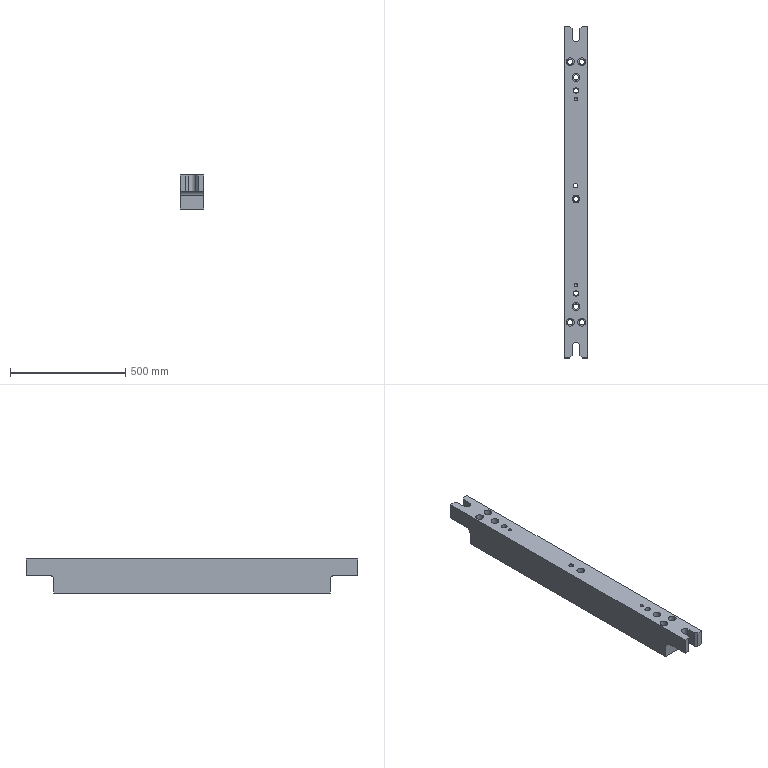Part | STEP file | lll_id2298_x_t | 1 solid | 56 faces | box 100 x 1440 x 147.5 mm | volume 18136196 mm3 | plane 29 | cylinder 25 | cone 2 | commonest cylinder face diameters 23.009 x7 34.008 x7 20 x3 14.506 x2 24 x2 34 x2
STEP:
#1=CARTESIAN_POINT('',(1317.435,-600.,222.5));
#2=VERTEX_POINT('',#1);
#3=CARTESIAN_POINT('',(1317.435,600.,222.5));
#4=VERTEX_POINT('',#3);
#5=CARTESIAN_POINT('',(1317.435,-1.,222.5));
#6=DIRECTION('',(0.,1.,0.));
#7=VECTOR('',#6,1.);
#8=LINE('',#5,#7);
#9=EDGE_CURVE('',#2,#4,#8,.T.);
#10=ORIENTED_EDGE('',*,*,#9,.T.);
#11=CARTESIAN_POINT('',(1417.435,600.,222.5));
#12=VERTEX_POINT('',#11);
#13=CARTESIAN_POINT('',(-848.88,600.,222.5));
#14=DIRECTION('',(1.,0.,0.));
#15=VECTOR('',#14,1.);
#16=LINE('',#13,#15);
#17=EDGE_CURVE('',#4,#12,#16,.T.);
#18=ORIENTED_EDGE('',*,*,#17,.T.);
#19=CARTESIAN_POINT('',(1417.435,-600.,222.5));
#20=VERTEX_POINT('',#19);
#21=CARTESIAN_POINT('',(1417.435,-1.,222.5));
#22=DIRECTION('',(0.,1.,0.));
#23=VECTOR('',#22,1.);
#24=LINE('',#21,#23);
#25=EDGE_CURVE('',#20,#12,#24,.T.);
#26=ORIENTED_EDGE('',*,*,#25,.F.);
#27=CARTESIAN_POINT('',(-848.88,-600.,222.5));
#28=DIRECTION('',(-1.,0.,0.));
#29=VECTOR('',#28,1.);
#30=LINE('',#27,#29);
#31=EDGE_CURVE('',#20,#2,#30,.T.);
#32=ORIENTED_EDGE('',*,*,#31,.T.);
#33=EDGE_LOOP('',(#10,#18,#26,#32));
#34=FACE_BOUND('',#33,.T.);
#35=CARTESIAN_POINT('',(1377.435,-440.,222.5));
#36=VERTEX_POINT('',#35);
#37=CARTESIAN_POINT('',(1367.435,-440.,222.5));
#38=DIRECTION('',(0.,0.,-1.));
#39=DIRECTION('',(1.,0.,0.));
#40=AXIS2_PLACEMENT_3D('',#37,#38,#39);
#41=CIRCLE('',#40,10.);
#42=EDGE_CURVE('',#36,#36,#41,.T.);
#43=ORIENTED_EDGE('',*,*,#42,.F.);
#44=EDGE_LOOP('',(#43));
#45=FACE_BOUND('',#44,.T.);
#46=CARTESIAN_POINT('',(1403.94,-565.,222.5));
#47=VERTEX_POINT('',#46);
#48=CARTESIAN_POINT('',(1392.435,-565.,222.5));
#49=DIRECTION('',(0.,0.,-1.));
#50=DIRECTION('',(1.,0.,0.));
#51=AXIS2_PLACEMENT_3D('',#48,#49,#50);
#52=CIRCLE('',#51,11.505);
#53=EDGE_CURVE('',#47,#47,#52,.T.);
#54=ORIENTED_EDGE('',*,*,#53,.F.);
#55=EDGE_LOOP('',(#54));
#56=FACE_BOUND('',#55,.T.);
#57=CARTESIAN_POINT('',(1353.94,-565.,222.5));
#58=VERTEX_POINT('',#57);
#59=CARTESIAN_POINT('',(1342.435,-565.,222.5));
#60=DIRECTION('',(0.,0.,-1.));
#61=DIRECTION('',(1.,0.,0.));
#62=AXIS2_PLACEMENT_3D('',#59,#60,#61);
#63=CIRCLE('',#62,11.505);
#64=EDGE_CURVE('',#58,#58,#63,.T.);
#65=ORIENTED_EDGE('',*,*,#64,.F.);
#66=EDGE_LOOP('',(#65));
#67=FACE_BOUND('',#66,.T.);
#68=CARTESIAN_POINT('',(1378.94,-497.,222.5));
#69=VERTEX_POINT('',#68);
#70=CARTESIAN_POINT('',(1367.435,-497.,222.5));
#71=DIRECTION('',(0.,0.,-1.));
#72=DIRECTION('',(1.,0.,0.));
#73=AXIS2_PLACEMENT_3D('',#70,#71,#72);
#74=CIRCLE('',#73,11.505);
#75=EDGE_CURVE('',#69,#69,#74,.T.);
#76=ORIENTED_EDGE('',*,*,#75,.F.);
#77=EDGE_LOOP('',(#76));
#78=FACE_BOUND('',#77,.T.);
#79=CARTESIAN_POINT('',(1378.94,-30.,222.5));
#80=VERTEX_POINT('',#79);
#81=CARTESIAN_POINT('',(1367.435,-30.,222.5));
#82=DIRECTION('',(0.,0.,-1.));
#83=DIRECTION('',(1.,0.,0.));
#84=AXIS2_PLACEMENT_3D('',#81,#82,#83);
#85=CIRCLE('',#84,11.505);
#86=EDGE_CURVE('',#80,#80,#85,.T.);
#87=ORIENTED_EDGE('',*,*,#86,.F.);
#88=EDGE_LOOP('',(#87));
#89=FACE_BOUND('',#88,.T.);
#90=CARTESIAN_POINT('',(1380.931,565.,222.5));
#91=VERTEX_POINT('',#90);
#92=CARTESIAN_POINT('',(1392.435,565.,222.5));
#93=DIRECTION('',(0.,0.,-1.));
#94=DIRECTION('',(-1.,0.,0.));
#95=AXIS2_PLACEMENT_3D('',#92,#93,#94);
#96=CIRCLE('',#95,11.505);
#97=EDGE_CURVE('',#91,#91,#96,.T.);
#98=ORIENTED_EDGE('',*,*,#97,.F.);
#99=EDGE_LOOP('',(#98));
#100=FACE_BOUND('',#99,.T.);
#101=CARTESIAN_POINT('',(1355.931,497.,222.5));
#102=VERTEX_POINT('',#101);
#103=CARTESIAN_POINT('',(1367.435,497.,222.5));
#104=DIRECTION('',(0.,0.,-1.));
#105=DIRECTION('',(-1.,0.,0.));
#106=AXIS2_PLACEMENT_3D('',#103,#104,#105);
#107=CIRCLE('',#106,11.505);
#108=EDGE_CURVE('',#102,#102,#107,.T.);
#109=ORIENTED_EDGE('',*,*,#108,.F.);
#110=EDGE_LOOP('',(#109));
#111=FACE_BOUND('',#110,.T.);
#112=CARTESIAN_POINT('',(1357.435,440.,222.5));
#113=VERTEX_POINT('',#112);
#114=CARTESIAN_POINT('',(1367.435,440.,222.5));
#115=DIRECTION('',(0.,0.,-1.));
#116=DIRECTION('',(-1.,0.,0.));
#117=AXIS2_PLACEMENT_3D('',#114,#115,#116);
#118=CIRCLE('',#117,10.);
#119=EDGE_CURVE('',#113,#113,#118,.T.);
#120=ORIENTED_EDGE('',*,*,#119,.F.);
#121=EDGE_LOOP('',(#120));
#122=FACE_BOUND('',#121,.T.);
#123=CARTESIAN_POINT('',(1330.931,565.,222.5));
#124=VERTEX_POINT('',#123);
#125=CARTESIAN_POINT('',(1342.435,565.,222.5));
#126=DIRECTION('',(0.,0.,-1.));
#127=DIRECTION('',(-1.,0.,0.));
#128=AXIS2_PLACEMENT_3D('',#125,#126,#127);
#129=CIRCLE('',#128,11.505);
#130=EDGE_CURVE('',#124,#124,#129,.T.);
#131=ORIENTED_EDGE('',*,*,#130,.F.);
#132=EDGE_LOOP('',(#131));
#133=FACE_BOUND('',#132,.T.);
#134=CARTESIAN_POINT('',(1376.,27.75,222.5));
#135=VERTEX_POINT('',#134);
#136=CARTESIAN_POINT('',(1366.,27.75,222.5));
#137=DIRECTION('',(0.,0.,1.));
#138=DIRECTION('',(1.,0.,0.));
#139=AXIS2_PLACEMENT_3D('',#136,#137,#138);
#140=CIRCLE('',#139,10.);
#141=EDGE_CURVE('',#135,#135,#140,.T.);
#142=ORIENTED_EDGE('',*,*,#141,.T.);
#143=EDGE_LOOP('',(#142));
#144=FACE_BOUND('',#143,.T.);
#145=CARTESIAN_POINT('',(-848.88,-1.,222.5));
#146=DIRECTION('',(0.,0.,-1.));
#147=DIRECTION('',(1.,0.,0.));
#148=AXIS2_PLACEMENT_3D('',#145,#146,#147);
#149=PLANE('',#148);
#150=ADVANCED_FACE('',(#34,#45,#56,#67,#78,#89,#100,#111,#122,#133,#144),#149,.T.);
#151=CARTESIAN_POINT('',(1356.,27.75,370.));
#152=VERTEX_POINT('',#151);
#153=CARTESIAN_POINT('',(1366.,27.75,370.));
#154=DIRECTION('',(0.,0.,-1.));
#155=DIRECTION('',(-1.,0.,0.));
#156=AXIS2_PLACEMENT_3D('',#153,#154,#155);
#157=CIRCLE('',#156,10.);
#158=EDGE_CURVE('',#152,#152,#157,.T.);
#159=ORIENTED_EDGE('',*,*,#158,.T.);
#160=EDGE_LOOP('',(#159));
#161=FACE_BOUND('',#160,.T.);
#162=CARTESIAN_POINT('',(1325.431,565.,370.));
#163=VERTEX_POINT('',#162);
#164=CARTESIAN_POINT('',(1342.435,565.,370.));
#165=DIRECTION('',(0.,0.,-1.));
#166=DIRECTION('',(-1.,0.,0.));
#167=AXIS2_PLACEMENT_3D('',#164,#165,#166);
#168=CIRCLE('',#167,17.004);
#169=EDGE_CURVE('',#163,#163,#168,.T.);
#170=ORIENTED_EDGE('',*,*,#169,.T.);
#171=EDGE_LOOP('',(#170));
#172=FACE_BOUND('',#171,.T.);
#173=CARTESIAN_POINT('',(1355.435,440.,370.));
#174=VERTEX_POINT('',#173);
#175=CARTESIAN_POINT('',(1367.435,440.,370.));
#176=DIRECTION('',(0.,0.,-1.));
#177=DIRECTION('',(-1.,0.,0.));
#178=AXIS2_PLACEMENT_3D('',#175,#176,#177);
#179=CIRCLE('',#178,12.);
#180=EDGE_CURVE('',#174,#174,#179,.T.);
#181=ORIENTED_EDGE('',*,*,#180,.T.);
#182=EDGE_LOOP('',(#181));
#183=FACE_BOUND('',#182,.T.);
#184=CARTESIAN_POINT('',(1350.431,497.,370.));
#185=VERTEX_POINT('',#184);
#186=CARTESIAN_POINT('',(1367.435,497.,370.));
#187=DIRECTION('',(0.,0.,-1.));
#188=DIRECTION('',(-1.,0.,0.));
#189=AXIS2_PLACEMENT_3D('',#186,#187,#188);
#190=CIRCLE('',#189,17.004);
#191=EDGE_CURVE('',#185,#185,#190,.T.);
#192=ORIENTED_EDGE('',*,*,#191,.T.);
#193=EDGE_LOOP('',(#192));
#194=FACE_BOUND('',#193,.T.);
#195=CARTESIAN_POINT('',(1375.431,565.,370.));
#196=VERTEX_POINT('',#195);
#197=CARTESIAN_POINT('',(1392.435,565.,370.));
#198=DIRECTION('',(0.,0.,-1.));
#199=DIRECTION('',(-1.,0.,0.));
#200=AXIS2_PLACEMENT_3D('',#197,#198,#199);
#201=CIRCLE('',#200,17.004);
#202=EDGE_CURVE('',#196,#196,#201,.T.);
#203=ORIENTED_EDGE('',*,*,#202,.T.);
#204=EDGE_LOOP('',(#203));
#205=FACE_BOUND('',#204,.T.);
#206=CARTESIAN_POINT('',(1384.439,-30.,370.));
#207=VERTEX_POINT('',#206);
#208=CARTESIAN_POINT('',(1367.435,-30.,370.));
#209=DIRECTION('',(0.,0.,-1.));
#210=DIRECTION('',(1.,0.,0.));
#211=AXIS2_PLACEMENT_3D('',#208,#209,#210);
#212=CIRCLE('',#211,17.004);
#213=EDGE_CURVE('',#207,#207,#212,.T.);
#214=ORIENTED_EDGE('',*,*,#213,.T.);
#215=EDGE_LOOP('',(#214));
#216=FACE_BOUND('',#215,.T.);
#217=CARTESIAN_POINT('',(1384.439,-497.,370.));
#218=VERTEX_POINT('',#217);
#219=CARTESIAN_POINT('',(1367.435,-497.,370.));
#220=DIRECTION('',(0.,0.,1.));
#221=DIRECTION('',(1.,0.,0.));
#222=AXIS2_PLACEMENT_3D('',#219,#220,#221);
#223=CIRCLE('',#222,17.004);
#224=EDGE_CURVE('',#218,#218,#223,.T.);
#225=ORIENTED_EDGE('',*,*,#224,.F.);
#226=EDGE_LOOP('',(#225));
#227=FACE_BOUND('',#226,.T.);
#228=CARTESIAN_POINT('',(1384.435,-710.,370.));
#229=VERTEX_POINT('',#228);
#230=CARTESIAN_POINT('',(1384.435,-670.,370.));
#231=VERTEX_POINT('',#230);
#232=CARTESIAN_POINT('',(1384.435,120.,370.));
#233=DIRECTION('',(0.,1.,0.));
#234=VECTOR('',#233,1.);
#235=LINE('',#232,#234);
#236=EDGE_CURVE('',#229,#231,#235,.T.);
#237=ORIENTED_EDGE('',*,*,#236,.F.);
#238=CARTESIAN_POINT('',(1394.435,-720.,370.));
#239=VERTEX_POINT('',#238);
#240=CARTESIAN_POINT('',(1384.435,-710.,370.));
#241=DIRECTION('',(0.7071,-0.7071,0.));
#242=VECTOR('',#241,1.);
#243=LINE('',#240,#242);
#244=EDGE_CURVE('',#229,#239,#243,.T.);
#245=ORIENTED_EDGE('',*,*,#244,.T.);
#246=CARTESIAN_POINT('',(1417.435,-720.,370.));
#247=VERTEX_POINT('',#246);
#248=CARTESIAN_POINT('',(-848.88,-720.,370.));
#249=DIRECTION('',(-1.,0.,0.));
#250=VECTOR('',#249,1.);
#251=LINE('',#248,#250);
#252=EDGE_CURVE('',#247,#239,#251,.T.);
#253=ORIENTED_EDGE('',*,*,#252,.F.);
#254=CARTESIAN_POINT('',(1417.435,720.,370.));
#255=VERTEX_POINT('',#254);
#256=CARTESIAN_POINT('',(1417.435,0.,370.));
#257=DIRECTION('',(0.,-1.,0.));
#258=VECTOR('',#257,1.);
#259=LINE('',#256,#258);
#260=EDGE_CURVE('',#255,#247,#259,.T.);
#261=ORIENTED_EDGE('',*,*,#260,.F.);
#262=CARTESIAN_POINT('',(1394.435,720.,370.));
#263=VERTEX_POINT('',#262);
#264=CARTESIAN_POINT('',(-848.88,720.,370.));
#265=DIRECTION('',(1.,0.,0.));
#266=VECTOR('',#265,1.);
#267=LINE('',#264,#266);
#268=EDGE_CURVE('',#263,#255,#267,.T.);
#269=ORIENTED_EDGE('',*,*,#268,.F.);
#270=CARTESIAN_POINT('',(1384.435,710.,370.));
#271=VERTEX_POINT('',#270);
#272=CARTESIAN_POINT('',(1350.935,676.5,370.));
#273=DIRECTION('',(0.7071,0.7071,0.));
#274=VECTOR('',#273,1.);
#275=LINE('',#272,#274);
#276=EDGE_CURVE('',#271,#263,#275,.T.);
#277=ORIENTED_EDGE('',*,*,#276,.F.);
#278=CARTESIAN_POINT('',(1384.435,670.,370.));
#279=VERTEX_POINT('',#278);
#280=CARTESIAN_POINT('',(1384.435,-120.,370.));
#281=DIRECTION('',(0.,-1.,0.));
#282=VECTOR('',#281,1.);
#283=LINE('',#280,#282);
#284=EDGE_CURVE('',#271,#279,#283,.T.);
#285=ORIENTED_EDGE('',*,*,#284,.T.);
#286=CARTESIAN_POINT('',(1350.435,670.,370.));
#287=VERTEX_POINT('',#286);
#288=CARTESIAN_POINT('',(1367.435,670.,370.));
#289=DIRECTION('',(0.,0.,-1.));
#290=DIRECTION('',(1.,0.,0.));
#291=AXIS2_PLACEMENT_3D('',#288,#289,#290);
#292=CIRCLE('',#291,17.);
#293=EDGE_CURVE('',#279,#287,#292,.T.);
#294=ORIENTED_EDGE('',*,*,#293,.T.);
#295=CARTESIAN_POINT('',(1350.435,710.,370.));
#296=VERTEX_POINT('',#295);
#297=CARTESIAN_POINT('',(1350.435,-120.,370.));
#298=DIRECTION('',(0.,1.,0.));
#299=VECTOR('',#298,1.);
#300=LINE('',#297,#299);
#301=EDGE_CURVE('',#287,#296,#300,.T.);
#302=ORIENTED_EDGE('',*,*,#301,.T.);
#303=CARTESIAN_POINT('',(1340.435,720.,370.));
#304=VERTEX_POINT('',#303);
#305=CARTESIAN_POINT('',(2043.935,16.5,370.));
#306=DIRECTION('',(0.7071,-0.7071,0.));
#307=VECTOR('',#306,1.);
#308=LINE('',#305,#307);
#309=EDGE_CURVE('',#304,#296,#308,.T.);
#310=ORIENTED_EDGE('',*,*,#309,.F.);
#311=CARTESIAN_POINT('',(1317.435,720.,370.));
#312=VERTEX_POINT('',#311);
#313=CARTESIAN_POINT('',(-848.88,720.,370.));
#314=DIRECTION('',(1.,0.,0.));
#315=VECTOR('',#314,1.);
#316=LINE('',#313,#315);
#317=EDGE_CURVE('',#312,#304,#316,.T.);
#318=ORIENTED_EDGE('',*,*,#317,.F.);
#319=CARTESIAN_POINT('',(1317.435,-720.,370.));
#320=VERTEX_POINT('',#319);
#321=CARTESIAN_POINT('',(1317.435,-1.,370.));
#322=DIRECTION('',(0.,1.,0.));
#323=VECTOR('',#322,1.);
#324=LINE('',#321,#323);
#325=EDGE_CURVE('',#320,#312,#324,.T.);
#326=ORIENTED_EDGE('',*,*,#325,.F.);
#327=CARTESIAN_POINT('',(1340.435,-720.,370.));
#328=VERTEX_POINT('',#327);
#329=CARTESIAN_POINT('',(-848.88,-720.,370.));
#330=DIRECTION('',(-1.,0.,0.));
#331=VECTOR('',#330,1.);
#332=LINE('',#329,#331);
#333=EDGE_CURVE('',#328,#320,#332,.T.);
#334=ORIENTED_EDGE('',*,*,#333,.F.);
#335=CARTESIAN_POINT('',(1350.435,-710.,370.));
#336=VERTEX_POINT('',#335);
#337=CARTESIAN_POINT('',(1350.435,-710.,370.));
#338=DIRECTION('',(0.7071,0.7071,0.));
#339=VECTOR('',#338,1.);
#340=LINE('',#337,#339);
#341=EDGE_CURVE('',#328,#336,#340,.T.);
#342=ORIENTED_EDGE('',*,*,#341,.T.);
#343=CARTESIAN_POINT('',(1350.435,-670.,370.));
#344=VERTEX_POINT('',#343);
#345=CARTESIAN_POINT('',(1350.435,120.,370.));
#346=DIRECTION('',(0.,-1.,0.));
#347=VECTOR('',#346,1.);
#348=LINE('',#345,#347);
#349=EDGE_CURVE('',#344,#336,#348,.T.);
#350=ORIENTED_EDGE('',*,*,#349,.F.);
#351=CARTESIAN_POINT('',(1367.435,-670.,370.));
#352=DIRECTION('',(0.,0.,1.));
#353=DIRECTION('',(1.,0.,0.));
#354=AXIS2_PLACEMENT_3D('',#351,#352,#353);
#355=CIRCLE('',#354,17.);
#356=EDGE_CURVE('',#231,#344,#355,.T.);
#357=ORIENTED_EDGE('',*,*,#356,.F.);
#358=EDGE_LOOP('',(#237,#245,#253,#261,#269,#277,#285,#294,#302,#310,#318,#326,#334,#342,#350,#357));
#359=FACE_BOUND('',#358,.T.);
#360=CARTESIAN_POINT('',(1355.435,-440.,370.));
#361=VERTEX_POINT('',#360);
#362=CARTESIAN_POINT('',(1367.435,-440.,370.));
#363=DIRECTION('',(0.,0.,-1.));
#364=DIRECTION('',(-1.,0.,0.));
#365=AXIS2_PLACEMENT_3D('',#362,#363,#364);
#366=CIRCLE('',#365,12.);
#367=EDGE_CURVE('',#361,#361,#366,.T.);
#368=ORIENTED_EDGE('',*,*,#367,.T.);
#369=EDGE_LOOP('',(#368));
#370=FACE_BOUND('',#369,.T.);
#371=CARTESIAN_POINT('',(1375.431,-565.,370.));
#372=VERTEX_POINT('',#371);
#373=CARTESIAN_POINT('',(1392.435,-565.,370.));
#374=DIRECTION('',(0.,0.,-1.));
#375=DIRECTION('',(-1.,0.,0.));
#376=AXIS2_PLACEMENT_3D('',#373,#374,#375);
#377=CIRCLE('',#376,17.004);
#378=EDGE_CURVE('',#372,#372,#377,.T.);
#379=ORIENTED_EDGE('',*,*,#378,.T.);
#380=EDGE_LOOP('',(#379));
#381=FACE_BOUND('',#380,.T.);
#382=CARTESIAN_POINT('',(1359.439,-565.,370.));
#383=VERTEX_POINT('',#382);
#384=CARTESIAN_POINT('',(1342.435,-565.,370.));
#385=DIRECTION('',(0.,0.,1.));
#386=DIRECTION('',(1.,0.,0.));
#387=AXIS2_PLACEMENT_3D('',#384,#385,#386);
#388=CIRCLE('',#387,17.004);
#389=EDGE_CURVE('',#383,#383,#388,.T.);
#390=ORIENTED_EDGE('',*,*,#389,.F.);
#391=EDGE_LOOP('',(#390));
#392=FACE_BOUND('',#391,.T.);
#393=CARTESIAN_POINT('',(1374.688,-403.,370.));
#394=VERTEX_POINT('',#393);
#395=CARTESIAN_POINT('',(1367.435,-403.,370.));
#396=DIRECTION('',(0.,0.,-1.));
#397=DIRECTION('',(1.,0.,0.));
#398=AXIS2_PLACEMENT_3D('',#395,#396,#397);
#399=CIRCLE('',#398,7.253);
#400=EDGE_CURVE('',#394,#394,#399,.T.);
#401=ORIENTED_EDGE('',*,*,#400,.T.);
#402=EDGE_LOOP('',(#401));
#403=FACE_BOUND('',#402,.T.);
#404=CARTESIAN_POINT('',(1374.688,403.,370.));
#405=VERTEX_POINT('',#404);
#406=CARTESIAN_POINT('',(1367.435,403.,370.));
#407=DIRECTION('',(0.,0.,1.));
#408=DIRECTION('',(1.,0.,0.));
#409=AXIS2_PLACEMENT_3D('',#406,#407,#408);
#410=CIRCLE('',#409,7.253);
#411=EDGE_CURVE('',#405,#405,#410,.T.);
#412=ORIENTED_EDGE('',*,*,#411,.F.);
#413=EDGE_LOOP('',(#412));
#414=FACE_BOUND('',#413,.T.);
#415=CARTESIAN_POINT('',(-848.88,-1.,370.));
#416=DIRECTION('',(0.,0.,-1.));
#417=DIRECTION('',(1.,0.,0.));
#418=AXIS2_PLACEMENT_3D('',#415,#416,#417);
#419=PLANE('',#418);
#420=ADVANCED_FACE('',(#161,#172,#183,#194,#205,#216,#227,#359,#370,#381,#392,#403,#414),#419,.F.);
#421=CARTESIAN_POINT('',(1417.435,600.,280.));
#422=VERTEX_POINT('',#421);
#423=CARTESIAN_POINT('',(1417.435,620.,300.));
#424=VERTEX_POINT('',#423);
#425=CARTESIAN_POINT('',(1417.435,620.,280.));
#426=DIRECTION('',(-1.,0.,0.));
#427=DIRECTION('',(0.,0.,-1.));
#428=AXIS2_PLACEMENT_3D('',#425,#426,#427);
#429=CIRCLE('',#428,20.);
#430=EDGE_CURVE('',#422,#424,#429,.T.);
#431=ORIENTED_EDGE('',*,*,#430,.F.);
#432=CARTESIAN_POINT('',(1317.435,600.,280.));
#433=VERTEX_POINT('',#432);
#434=CARTESIAN_POINT('',(1407.435,600.,280.));
#435=DIRECTION('',(1.,0.,0.));
#436=VECTOR('',#435,1.);
#437=LINE('',#434,#436);
#438=EDGE_CURVE('',#433,#422,#437,.T.);
#439=ORIENTED_EDGE('',*,*,#438,.F.);
#440=CARTESIAN_POINT('',(1317.435,620.,300.));
#441=VERTEX_POINT('',#440);
#442=CARTESIAN_POINT('',(1317.435,620.,280.));
#443=DIRECTION('',(1.,0.,0.));
#444=DIRECTION('',(0.,0.,-1.));
#445=AXIS2_PLACEMENT_3D('',#442,#443,#444);
#446=CIRCLE('',#445,20.);
#447=EDGE_CURVE('',#441,#433,#446,.T.);
#448=ORIENTED_EDGE('',*,*,#447,.F.);
#449=CARTESIAN_POINT('',(1327.435,620.,300.));
#450=DIRECTION('',(-1.,0.,0.));
#451=VECTOR('',#450,1.);
#452=LINE('',#449,#451);
#453=EDGE_CURVE('',#424,#441,#452,.T.);
#454=ORIENTED_EDGE('',*,*,#453,.F.);
#455=EDGE_LOOP('',(#431,#439,#448,#454));
#456=FACE_OUTER_BOUND('',#455,.T.);
#457=CARTESIAN_POINT('',(1367.435,620.,280.));
#458=DIRECTION('',(1.,0.,0.));
#459=DIRECTION('',(0.,0.,1.));
#460=AXIS2_PLACEMENT_3D('',#457,#458,#459);
#461=CYLINDRICAL_SURFACE('',#460,20.);
#462=ADVANCED_FACE('',(#456),#461,.F.);
#463=CARTESIAN_POINT('',(1417.435,720.,300.));
#464=VERTEX_POINT('',#463);
#465=CARTESIAN_POINT('',(1417.435,-641.5,300.));
#466=DIRECTION('',(0.,1.,0.));
#467=VECTOR('',#466,1.);
#468=LINE('',#465,#467);
#469=EDGE_CURVE('',#424,#464,#468,.T.);
#470=ORIENTED_EDGE('',*,*,#469,.F.);
#471=ORIENTED_EDGE('',*,*,#453,.T.);
#472=CARTESIAN_POINT('',(1317.435,720.,300.));
#473=VERTEX_POINT('',#472);
#474=CARTESIAN_POINT('',(1317.435,-641.5,300.));
#475=DIRECTION('',(0.,1.,0.));
#476=VECTOR('',#475,1.);
#477=LINE('',#474,#476);
#478=EDGE_CURVE('',#441,#473,#477,.T.);
#479=ORIENTED_EDGE('',*,*,#478,.T.);
#480=CARTESIAN_POINT('',(1340.435,720.,300.));
#481=VERTEX_POINT('',#480);
#482=CARTESIAN_POINT('',(1367.435,720.,300.));
#483=DIRECTION('',(1.,0.,0.));
#484=VECTOR('',#483,1.);
#485=LINE('',#482,#484);
#486=EDGE_CURVE('',#473,#481,#485,.T.);
#487=ORIENTED_EDGE('',*,*,#486,.T.);
#488=CARTESIAN_POINT('',(1350.435,710.,300.));
#489=VERTEX_POINT('',#488);
#490=CARTESIAN_POINT('',(1340.435,720.,300.));
#491=DIRECTION('',(0.7071,-0.7071,0.));
#492=VECTOR('',#491,1.);
#493=LINE('',#490,#492);
#494=EDGE_CURVE('',#481,#489,#493,.T.);
#495=ORIENTED_EDGE('',*,*,#494,.T.);
#496=CARTESIAN_POINT('',(1350.435,670.,300.));
#497=VERTEX_POINT('',#496);
#498=CARTESIAN_POINT('',(1350.435,-641.5,300.));
#499=DIRECTION('',(0.,-1.,0.));
#500=VECTOR('',#499,1.);
#501=LINE('',#498,#500);
#502=EDGE_CURVE('',#489,#497,#501,.T.);
#503=ORIENTED_EDGE('',*,*,#502,.T.);
#504=CARTESIAN_POINT('',(1384.435,670.,300.));
#505=VERTEX_POINT('',#504);
#506=CARTESIAN_POINT('',(1367.435,670.,300.));
#507=DIRECTION('',(0.,0.,-1.));
#508=DIRECTION('',(-1.,0.,0.));
#509=AXIS2_PLACEMENT_3D('',#506,#507,#508);
#510=CIRCLE('',#509,17.);
#511=EDGE_CURVE('',#505,#497,#510,.T.);
#512=ORIENTED_EDGE('',*,*,#511,.F.);
#513=CARTESIAN_POINT('',(1384.435,710.,300.));
#514=VERTEX_POINT('',#513);
#515=CARTESIAN_POINT('',(1384.435,-641.5,300.));
#516=DIRECTION('',(0.,1.,0.));
#517=VECTOR('',#516,1.);
#518=LINE('',#515,#517);
#519=EDGE_CURVE('',#505,#514,#518,.T.);
#520=ORIENTED_EDGE('',*,*,#519,.T.);
#521=CARTESIAN_POINT('',(1394.435,720.,300.));
#522=VERTEX_POINT('',#521);
#523=CARTESIAN_POINT('',(1394.435,720.,300.));
#524=DIRECTION('',(0.7071,0.7071,0.));
#525=VECTOR('',#524,1.);
#526=LINE('',#523,#525);
#527=EDGE_CURVE('',#514,#522,#526,.T.);
#528=ORIENTED_EDGE('',*,*,#527,.T.);
#529=CARTESIAN_POINT('',(1367.435,720.,300.));
#530=DIRECTION('',(1.,0.,0.));
#531=VECTOR('',#530,1.);
#532=LINE('',#529,#531);
#533=EDGE_CURVE('',#522,#464,#532,.T.);
#534=ORIENTED_EDGE('',*,*,#533,.T.);
#535=EDGE_LOOP('',(#470,#471,#479,#487,#495,#503,#512,#520,#528,#534));
#536=FACE_OUTER_BOUND('',#535,.T.);
#537=CARTESIAN_POINT('',(1367.435,-641.5,300.));
#538=DIRECTION('',(0.,0.,-1.));
#539=DIRECTION('',(1.,0.,0.));
#540=AXIS2_PLACEMENT_3D('',#537,#538,#539);
#541=PLANE('',#540);
#542=ADVANCED_FACE('',(#536),#541,.T.);
#543=CARTESIAN_POINT('',(1417.435,-720.,300.));
#544=VERTEX_POINT('',#543);
#545=CARTESIAN_POINT('',(1394.435,-720.,300.));
#546=VERTEX_POINT('',#545);
#547=CARTESIAN_POINT('',(1367.435,-720.,300.));
#548=DIRECTION('',(-1.,0.,0.));
#549=VECTOR('',#548,1.);
#550=LINE('',#547,#549);
#551=EDGE_CURVE('',#544,#546,#550,.T.);
#552=ORIENTED_EDGE('',*,*,#551,.T.);
#553=CARTESIAN_POINT('',(1384.435,-710.,300.));
#554=VERTEX_POINT('',#553);
#555=CARTESIAN_POINT('',(1361.685,-687.25,300.));
#556=DIRECTION('',(-0.7071,0.7071,0.));
#557=VECTOR('',#556,1.);
#558=LINE('',#555,#557);
#559=EDGE_CURVE('',#546,#554,#558,.T.);
#560=ORIENTED_EDGE('',*,*,#559,.T.);
#561=CARTESIAN_POINT('',(1384.435,-670.,300.));
#562=VERTEX_POINT('',#561);
#563=CARTESIAN_POINT('',(1384.435,-661.5,300.));
#564=DIRECTION('',(0.,-1.,0.));
#565=VECTOR('',#564,1.);
#566=LINE('',#563,#565);
#567=EDGE_CURVE('',#562,#554,#566,.T.);
#568=ORIENTED_EDGE('',*,*,#567,.F.);
#569=CARTESIAN_POINT('',(1350.435,-670.,300.));
#570=VERTEX_POINT('',#569);
#571=CARTESIAN_POINT('',(1367.435,-670.,300.));
#572=DIRECTION('',(0.,0.,1.));
#573=DIRECTION('',(1.,0.,0.));
#574=AXIS2_PLACEMENT_3D('',#571,#572,#573);
#575=CIRCLE('',#574,17.);
#576=EDGE_CURVE('',#562,#570,#575,.T.);
#577=ORIENTED_EDGE('',*,*,#576,.T.);
#578=CARTESIAN_POINT('',(1350.435,-710.,300.));
#579=VERTEX_POINT('',#578);
#580=CARTESIAN_POINT('',(1350.435,-661.5,300.));
#581=DIRECTION('',(0.,1.,0.));
#582=VECTOR('',#581,1.);
#583=LINE('',#580,#582);
#584=EDGE_CURVE('',#579,#570,#583,.T.);
#585=ORIENTED_EDGE('',*,*,#584,.F.);
#586=CARTESIAN_POINT('',(1340.435,-720.,300.));
#587=VERTEX_POINT('',#586);
#588=CARTESIAN_POINT('',(1373.185,-687.25,300.));
#589=DIRECTION('',(-0.7071,-0.7071,0.));
#590=VECTOR('',#589,1.);
#591=LINE('',#588,#590);
#592=EDGE_CURVE('',#579,#587,#591,.T.);
#593=ORIENTED_EDGE('',*,*,#592,.T.);
#594=CARTESIAN_POINT('',(1317.435,-720.,300.));
#595=VERTEX_POINT('',#594);
#596=CARTESIAN_POINT('',(1367.435,-720.,300.));
#597=DIRECTION('',(-1.,0.,0.));
#598=VECTOR('',#597,1.);
#599=LINE('',#596,#598);
#600=EDGE_CURVE('',#587,#595,#599,.T.);
#601=ORIENTED_EDGE('',*,*,#600,.T.);
#602=CARTESIAN_POINT('',(1317.435,-620.,300.));
#603=VERTEX_POINT('',#602);
#604=CARTESIAN_POINT('',(1317.435,-681.5,300.));
#605=DIRECTION('',(0.,1.,0.));
#606=VECTOR('',#605,1.);
#607=LINE('',#604,#606);
#608=EDGE_CURVE('',#595,#603,#607,.T.);
#609=ORIENTED_EDGE('',*,*,#608,.T.);
#610=CARTESIAN_POINT('',(1417.435,-620.,300.));
#611=VERTEX_POINT('',#610);
#612=CARTESIAN_POINT('',(1407.435,-620.,300.));
#613=DIRECTION('',(1.,0.,0.));
#614=VECTOR('',#613,1.);
#615=LINE('',#612,#614);
#616=EDGE_CURVE('',#603,#611,#615,.T.);
#617=ORIENTED_EDGE('',*,*,#616,.T.);
#618=CARTESIAN_POINT('',(1417.435,-681.5,300.));
#619=DIRECTION('',(0.,1.,0.));
#620=VECTOR('',#619,1.);
#621=LINE('',#618,#620);
#622=EDGE_CURVE('',#544,#611,#621,.T.);
#623=ORIENTED_EDGE('',*,*,#622,.F.);
#624=EDGE_LOOP('',(#552,#560,#568,#577,#585,#593,#601,#609,#617,#623));
#625=FACE_OUTER_BOUND('',#624,.T.);
#626=CARTESIAN_POINT('',(1367.435,-681.5,300.));
#627=DIRECTION('',(0.,0.,-1.));
#628=DIRECTION('',(1.,0.,0.));
#629=AXIS2_PLACEMENT_3D('',#626,#627,#628);
#630=PLANE('',#629);
#631=ADVANCED_FACE('',(#625),#630,.T.);
#632=CARTESIAN_POINT('',(1317.435,-600.,280.));
#633=VERTEX_POINT('',#632);
#634=CARTESIAN_POINT('',(1317.435,-620.,280.));
#635=DIRECTION('',(1.,0.,0.));
#636=DIRECTION('',(0.,0.,-1.));
#637=AXIS2_PLACEMENT_3D('',#634,#635,#636);
#638=CIRCLE('',#637,20.);
#639=EDGE_CURVE('',#633,#603,#638,.T.);
#640=ORIENTED_EDGE('',*,*,#639,.F.);
#641=CARTESIAN_POINT('',(1417.435,-600.,280.));
#642=VERTEX_POINT('',#641);
#643=CARTESIAN_POINT('',(1327.435,-600.,280.));
#644=DIRECTION('',(-1.,0.,0.));
#645=VECTOR('',#644,1.);
#646=LINE('',#643,#645);
#647=EDGE_CURVE('',#642,#633,#646,.T.);
#648=ORIENTED_EDGE('',*,*,#647,.F.);
#649=CARTESIAN_POINT('',(1417.435,-620.,280.));
#650=DIRECTION('',(-1.,0.,0.));
#651=DIRECTION('',(0.,0.,-1.));
#652=AXIS2_PLACEMENT_3D('',#649,#650,#651);
#653=CIRCLE('',#652,20.);
#654=EDGE_CURVE('',#611,#642,#653,.T.);
#655=ORIENTED_EDGE('',*,*,#654,.F.);
#656=ORIENTED_EDGE('',*,*,#616,.F.);
#657=EDGE_LOOP('',(#640,#648,#655,#656));
#658=FACE_OUTER_BOUND('',#657,.T.);
#659=CARTESIAN_POINT('',(1367.435,-620.,280.));
#660=DIRECTION('',(-1.,0.,0.));
#661=DIRECTION('',(0.,0.,-1.));
#662=AXIS2_PLACEMENT_3D('',#659,#660,#661);
#663=CYLINDRICAL_SURFACE('',#662,20.);
#664=ADVANCED_FACE('',(#658),#663,.F.);
#665=CARTESIAN_POINT('',(1355.435,-440.,270.));
#666=VERTEX_POINT('',#665);
#667=CARTESIAN_POINT('',(1367.435,-440.,270.));
#668=DIRECTION('',(0.,0.,-1.));
#669=DIRECTION('',(-1.,0.,0.));
#670=AXIS2_PLACEMENT_3D('',#667,#668,#669);
#671=CIRCLE('',#670,12.);
#672=EDGE_CURVE('',#666,#666,#671,.T.);
#673=ORIENTED_EDGE('',*,*,#672,.F.);
#674=EDGE_LOOP('',(#673));
#675=FACE_BOUND('',#674,.T.);
#676=CARTESIAN_POINT('',(1377.435,-440.,270.));
#677=VERTEX_POINT('',#676);
#678=CARTESIAN_POINT('',(1367.435,-440.,270.));
#679=DIRECTION('',(0.,0.,1.));
#680=DIRECTION('',(1.,0.,0.));
#681=AXIS2_PLACEMENT_3D('',#678,#679,#680);
#682=CIRCLE('',#681,10.);
#683=EDGE_CURVE('',#677,#677,#682,.T.);
#684=ORIENTED_EDGE('',*,*,#683,.F.);
#685=EDGE_LOOP('',(#684));
#686=FACE_BOUND('',#685,.T.);
#687=CARTESIAN_POINT('',(1367.435,-440.,270.));
#688=DIRECTION('',(0.,0.,-1.));
#689=DIRECTION('',(1.,0.,0.));
#690=AXIS2_PLACEMENT_3D('',#687,#688,#689);
#691=PLANE('',#690);
#692=ADVANCED_FACE('',(#675,#686),#691,.F.);
#693=CARTESIAN_POINT('',(1403.94,-565.,272.5));
#694=VERTEX_POINT('',#693);
#695=CARTESIAN_POINT('',(1392.435,-565.,272.5));
#696=DIRECTION('',(0.,0.,-1.));
#697=DIRECTION('',(1.,0.,0.));
#698=AXIS2_PLACEMENT_3D('',#695,#696,#697);
#699=CIRCLE('',#698,11.505);
#700=EDGE_CURVE('',#694,#694,#699,.T.);
#701=ORIENTED_EDGE('',*,*,#700,.T.);
#702=EDGE_LOOP('',(#701));
#703=FACE_BOUND('',#702,.T.);
#704=CARTESIAN_POINT('',(1375.431,-565.,272.5));
#705=VERTEX_POINT('',#704);
#706=CARTESIAN_POINT('',(1392.435,-565.,272.5));
#707=DIRECTION('',(0.,0.,-1.));
#708=DIRECTION('',(-1.,0.,0.));
#709=AXIS2_PLACEMENT_3D('',#706,#707,#708);
#710=CIRCLE('',#709,17.004);
#711=EDGE_CURVE('',#705,#705,#710,.T.);
#712=ORIENTED_EDGE('',*,*,#711,.F.);
#713=EDGE_LOOP('',(#712));
#714=FACE_BOUND('',#713,.T.);
#715=CARTESIAN_POINT('',(1392.435,-565.,272.5));
#716=DIRECTION('',(0.,0.,-1.));
#717=DIRECTION('',(1.,0.,0.));
#718=AXIS2_PLACEMENT_3D('',#715,#716,#717);
#719=PLANE('',#718);
#720=ADVANCED_FACE('',(#703,#714),#719,.F.);
#721=CARTESIAN_POINT('',(1330.931,-565.,272.5));
#722=VERTEX_POINT('',#721);
#723=CARTESIAN_POINT('',(1342.435,-565.,272.5));
#724=DIRECTION('',(0.,0.,1.));
#725=DIRECTION('',(-1.,0.,0.));
#726=AXIS2_PLACEMENT_3D('',#723,#724,#725);
#727=CIRCLE('',#726,11.505);
#728=EDGE_CURVE('',#722,#722,#727,.T.);
#729=ORIENTED_EDGE('',*,*,#728,.F.);
#730=EDGE_LOOP('',(#729));
#731=FACE_BOUND('',#730,.T.);
#732=CARTESIAN_POINT('',(1359.439,-565.,272.5));
#733=VERTEX_POINT('',#732);
#734=CARTESIAN_POINT('',(1342.435,-565.,272.5));
#735=DIRECTION('',(0.,0.,1.));
#736=DIRECTION('',(1.,0.,0.));
#737=AXIS2_PLACEMENT_3D('',#734,#735,#736);
#738=CIRCLE('',#737,17.004);
#739=EDGE_CURVE('',#733,#733,#738,.T.);
#740=ORIENTED_EDGE('',*,*,#739,.T.);
#741=EDGE_LOOP('',(#740));
#742=FACE_BOUND('',#741,.T.);
#743=CARTESIAN_POINT('',(1342.435,-565.,272.5));
#744=DIRECTION('',(0.,0.,-1.));
#745=DIRECTION('',(-1.,0.,0.));
#746=AXIS2_PLACEMENT_3D('',#743,#744,#745);
#747=PLANE('',#746);
#748=ADVANCED_FACE('',(#731,#742),#747,.F.);
#749=CARTESIAN_POINT('',(1355.931,-497.,272.5));
#750=VERTEX_POINT('',#749);
#751=CARTESIAN_POINT('',(1367.435,-497.,272.5));
#752=DIRECTION('',(0.,0.,1.));
#753=DIRECTION('',(-1.,0.,0.));
#754=AXIS2_PLACEMENT_3D('',#751,#752,#753);
#755=CIRCLE('',#754,11.505);
#756=EDGE_CURVE('',#750,#750,#755,.T.);
#757=ORIENTED_EDGE('',*,*,#756,.F.);
#758=EDGE_LOOP('',(#757));
#759=FACE_BOUND('',#758,.T.);
#760=CARTESIAN_POINT('',(1384.439,-497.,272.5));
#761=VERTEX_POINT('',#760);
#762=CARTESIAN_POINT('',(1367.435,-497.,272.5));
#763=DIRECTION('',(0.,0.,1.));
#764=DIRECTION('',(1.,0.,0.));
#765=AXIS2_PLACEMENT_3D('',#762,#763,#764);
#766=CIRCLE('',#765,17.004);
#767=EDGE_CURVE('',#761,#761,#766,.T.);
#768=ORIENTED_EDGE('',*,*,#767,.T.);
#769=EDGE_LOOP('',(#768));
#770=FACE_BOUND('',#769,.T.);
#771=CARTESIAN_POINT('',(1367.435,-497.,272.5));
#772=DIRECTION('',(0.,0.,-1.));
#773=DIRECTION('',(-1.,0.,0.));
#774=AXIS2_PLACEMENT_3D('',#771,#772,#773);
#775=PLANE('',#774);
#776=ADVANCED_FACE('',(#759,#770),#775,.F.);
#777=CARTESIAN_POINT('',(1355.931,-30.,272.5));
#778=VERTEX_POINT('',#777);
#779=CARTESIAN_POINT('',(1367.435,-30.,272.5));
#780=DIRECTION('',(0.,0.,-1.));
#781=DIRECTION('',(-1.,0.,0.));
#782=AXIS2_PLACEMENT_3D('',#779,#780,#781);
#783=CIRCLE('',#782,11.505);
#784=EDGE_CURVE('',#778,#778,#783,.T.);
#785=ORIENTED_EDGE('',*,*,#784,.T.);
#786=EDGE_LOOP('',(#785));
#787=FACE_BOUND('',#786,.T.);
#788=CARTESIAN_POINT('',(1384.439,-30.,272.5));
#789=VERTEX_POINT('',#788);
#790=CARTESIAN_POINT('',(1367.435,-30.,272.5));
#791=DIRECTION('',(0.,0.,-1.));
#792=DIRECTION('',(1.,0.,0.));
#793=AXIS2_PLACEMENT_3D('',#790,#791,#792);
#794=CIRCLE('',#793,17.004);
#795=EDGE_CURVE('',#789,#789,#794,.T.);
#796=ORIENTED_EDGE('',*,*,#795,.F.);
#797=EDGE_LOOP('',(#796));
#798=FACE_BOUND('',#797,.T.);
#799=CARTESIAN_POINT('',(1367.435,-10.,272.5));
#800=DIRECTION('',(0.,0.,-1.));
#801=DIRECTION('',(-1.,0.,0.));
#802=AXIS2_PLACEMENT_3D('',#799,#800,#801);
#803=PLANE('',#802);
#804=ADVANCED_FACE('',(#787,#798),#803,.F.);
#805=ORIENTED_EDGE('',*,*,#739,.F.);
#806=EDGE_LOOP('',(#805));
#807=FACE_BOUND('',#806,.T.);
#808=ORIENTED_EDGE('',*,*,#389,.T.);
#809=EDGE_LOOP('',(#808));
#810=FACE_BOUND('',#809,.T.);
#811=CARTESIAN_POINT('',(1342.435,-565.,370.));
#812=DIRECTION('',(0.,0.,-1.));
#813=DIRECTION('',(1.,0.,0.));
#814=AXIS2_PLACEMENT_3D('',#811,#812,#813);
#815=CYLINDRICAL_SURFACE('',#814,17.004);
#816=ADVANCED_FACE('',(#807,#810),#815,.F.);
#817=ORIENTED_EDGE('',*,*,#711,.T.);
#818=EDGE_LOOP('',(#817));
#819=FACE_BOUND('',#818,.T.);
#820=ORIENTED_EDGE('',*,*,#378,.F.);
#821=EDGE_LOOP('',(#820));
#822=FACE_BOUND('',#821,.T.);
#823=CARTESIAN_POINT('',(1392.435,-565.,370.));
#824=DIRECTION('',(0.,0.,-1.));
#825=DIRECTION('',(-1.,0.,0.));
#826=AXIS2_PLACEMENT_3D('',#823,#824,#825);
#827=CYLINDRICAL_SURFACE('',#826,17.004);
#828=ADVANCED_FACE('',(#819,#822),#827,.F.);
#829=ORIENTED_EDGE('',*,*,#672,.T.);
#830=EDGE_LOOP('',(#829));
#831=FACE_BOUND('',#830,.T.);
#832=ORIENTED_EDGE('',*,*,#367,.F.);
#833=EDGE_LOOP('',(#832));
#834=FACE_BOUND('',#833,.T.);
#835=CARTESIAN_POINT('',(1367.435,-440.,370.));
#836=DIRECTION('',(0.,0.,-1.));
#837=DIRECTION('',(-1.,0.,0.));
#838=AXIS2_PLACEMENT_3D('',#835,#836,#837);
#839=CYLINDRICAL_SURFACE('',#838,12.);
#840=ADVANCED_FACE('',(#831,#834),#839,.F.);
#841=ORIENTED_EDGE('',*,*,#301,.F.);
#842=CARTESIAN_POINT('',(1350.435,670.,370.));
#843=DIRECTION('',(0.,0.,-1.));
#844=VECTOR('',#843,1.);
#845=LINE('',#842,#844);
#846=EDGE_CURVE('',#287,#497,#845,.T.);
#847=ORIENTED_EDGE('',*,*,#846,.T.);
#848=ORIENTED_EDGE('',*,*,#502,.F.);
#849=CARTESIAN_POINT('',(1350.435,710.,385.));
#850=DIRECTION('',(0.,0.,-1.));
#851=VECTOR('',#850,1.);
#852=LINE('',#849,#851);
#853=EDGE_CURVE('',#296,#489,#852,.T.);
#854=ORIENTED_EDGE('',*,*,#853,.F.);
#855=EDGE_LOOP('',(#841,#847,#848,#854));
#856=FACE_OUTER_BOUND('',#855,.T.);
#857=CARTESIAN_POINT('',(1350.435,-720.,385.));
#858=DIRECTION('',(1.,0.,0.));
#859=DIRECTION('',(0.,0.,-1.));
#860=AXIS2_PLACEMENT_3D('',#857,#858,#859);
#861=PLANE('',#860);
#862=ADVANCED_FACE('',(#856),#861,.T.);
#863=ORIENTED_EDGE('',*,*,#846,.F.);
#864=ORIENTED_EDGE('',*,*,#293,.F.);
#865=CARTESIAN_POINT('',(1384.435,670.,370.));
#866=DIRECTION('',(0.,0.,1.));
#867=VECTOR('',#866,1.);
#868=LINE('',#865,#867);
#869=EDGE_CURVE('',#505,#279,#868,.T.);
#870=ORIENTED_EDGE('',*,*,#869,.F.);
#871=ORIENTED_EDGE('',*,*,#511,.T.);
#872=EDGE_LOOP('',(#863,#864,#870,#871));
#873=FACE_OUTER_BOUND('',#872,.T.);
#874=CARTESIAN_POINT('',(1367.435,670.,345.));
#875=DIRECTION('',(0.,0.,-1.));
#876=DIRECTION('',(-1.,0.,0.));
#877=AXIS2_PLACEMENT_3D('',#874,#875,#876);
#878=CYLINDRICAL_SURFACE('',#877,17.);
#879=ADVANCED_FACE('',(#873),#878,.F.);
#880=ORIENTED_EDGE('',*,*,#519,.F.);
#881=ORIENTED_EDGE('',*,*,#869,.T.);
#882=ORIENTED_EDGE('',*,*,#284,.F.);
#883=CARTESIAN_POINT('',(1384.435,710.,385.));
#884=DIRECTION('',(0.,0.,1.));
#885=VECTOR('',#884,1.);
#886=LINE('',#883,#885);
#887=EDGE_CURVE('',#514,#271,#886,.T.);
#888=ORIENTED_EDGE('',*,*,#887,.F.);
#889=EDGE_LOOP('',(#880,#881,#882,#888));
#890=FACE_OUTER_BOUND('',#889,.T.);
#891=CARTESIAN_POINT('',(1384.435,-720.,385.));
#892=DIRECTION('',(-1.,0.,0.));
#893=DIRECTION('',(0.,0.,1.));
#894=AXIS2_PLACEMENT_3D('',#891,#892,#893);
#895=PLANE('',#894);
#896=ADVANCED_FACE('',(#890),#895,.T.);
#897=ORIENTED_EDGE('',*,*,#276,.T.);
#898=CARTESIAN_POINT('',(1394.435,720.,-450.));
#899=DIRECTION('',(0.,0.,-1.));
#900=VECTOR('',#899,1.);
#901=LINE('',#898,#900);
#902=EDGE_CURVE('',#263,#522,#901,.T.);
#903=ORIENTED_EDGE('',*,*,#902,.T.);
#904=ORIENTED_EDGE('',*,*,#527,.F.);
#905=ORIENTED_EDGE('',*,*,#887,.T.);
#906=EDGE_LOOP('',(#897,#903,#904,#905));
#907=FACE_OUTER_BOUND('',#906,.T.);
#908=CARTESIAN_POINT('',(1394.435,720.,-450.));
#909=DIRECTION('',(0.7071,-0.7071,0.));
#910=DIRECTION('',(0.,0.,-1.));
#911=AXIS2_PLACEMENT_3D('',#908,#909,#910);
#912=PLANE('',#911);
#913=ADVANCED_FACE('',(#907),#912,.F.);
#914=ORIENTED_EDGE('',*,*,#902,.F.);
#915=ORIENTED_EDGE('',*,*,#268,.T.);
#916=CARTESIAN_POINT('',(1417.435,720.,241.25));
#917=DIRECTION('',(0.,0.,-1.));
#918=VECTOR('',#917,1.);
#919=LINE('',#916,#918);
#920=EDGE_CURVE('',#255,#464,#919,.T.);
#921=ORIENTED_EDGE('',*,*,#920,.T.);
#922=ORIENTED_EDGE('',*,*,#533,.F.);
#923=EDGE_LOOP('',(#914,#915,#921,#922));
#924=FACE_OUTER_BOUND('',#923,.T.);
#925=CARTESIAN_POINT('',(1337.435,720.,310.));
#926=DIRECTION('',(0.,1.,0.));
#927=DIRECTION('',(0.,0.,-1.));
#928=AXIS2_PLACEMENT_3D('',#925,#926,#927);
#929=PLANE('',#928);
#930=ADVANCED_FACE('',(#924),#929,.T.);
#931=ORIENTED_EDGE('',*,*,#252,.T.);
#932=CARTESIAN_POINT('',(1394.435,-720.,310.));
#933=DIRECTION('',(0.,0.,-1.));
#934=VECTOR('',#933,1.);
#935=LINE('',#932,#934);
#936=EDGE_CURVE('',#239,#546,#935,.T.);
#937=ORIENTED_EDGE('',*,*,#936,.T.);
#938=ORIENTED_EDGE('',*,*,#551,.F.);
#939=CARTESIAN_POINT('',(1417.435,-720.,241.25));
#940=DIRECTION('',(0.,0.,1.));
#941=VECTOR('',#940,1.);
#942=LINE('',#939,#941);
#943=EDGE_CURVE('',#544,#247,#942,.T.);
#944=ORIENTED_EDGE('',*,*,#943,.T.);
#945=EDGE_LOOP('',(#931,#937,#938,#944));
#946=FACE_OUTER_BOUND('',#945,.T.);
#947=CARTESIAN_POINT('',(5307.435,-720.,310.));
#948=DIRECTION('',(0.,-1.,0.));
#949=DIRECTION('',(0.,0.,1.));
#950=AXIS2_PLACEMENT_3D('',#947,#948,#949);
#951=PLANE('',#950);
#952=ADVANCED_FACE('',(#946),#951,.T.);
#953=ORIENTED_EDGE('',*,*,#567,.T.);
#954=CARTESIAN_POINT('',(1384.435,-710.,385.));
#955=DIRECTION('',(0.,0.,1.));
#956=VECTOR('',#955,1.);
#957=LINE('',#954,#956);
#958=EDGE_CURVE('',#554,#229,#957,.T.);
#959=ORIENTED_EDGE('',*,*,#958,.T.);
#960=ORIENTED_EDGE('',*,*,#236,.T.);
#961=CARTESIAN_POINT('',(1384.435,-670.,370.));
#962=DIRECTION('',(0.,0.,1.));
#963=VECTOR('',#962,1.);
#964=LINE('',#961,#963);
#965=EDGE_CURVE('',#562,#231,#964,.T.);
#966=ORIENTED_EDGE('',*,*,#965,.F.);
#967=EDGE_LOOP('',(#953,#959,#960,#966));
#968=FACE_OUTER_BOUND('',#967,.T.);
#969=CARTESIAN_POINT('',(1384.435,720.,385.));
#970=DIRECTION('',(-1.,0.,0.));
#971=DIRECTION('',(0.,0.,1.));
#972=AXIS2_PLACEMENT_3D('',#969,#970,#971);
#973=PLANE('',#972);
#974=ADVANCED_FACE('',(#968),#973,.T.);
#975=CARTESIAN_POINT('',(1350.435,-670.,370.));
#976=DIRECTION('',(0.,0.,-1.));
#977=VECTOR('',#976,1.);
#978=LINE('',#975,#977);
#979=EDGE_CURVE('',#344,#570,#978,.T.);
#980=ORIENTED_EDGE('',*,*,#979,.T.);
#981=ORIENTED_EDGE('',*,*,#576,.F.);
#982=ORIENTED_EDGE('',*,*,#965,.T.);
#983=ORIENTED_EDGE('',*,*,#356,.T.);
#984=EDGE_LOOP('',(#980,#981,#982,#983));
#985=FACE_OUTER_BOUND('',#984,.T.);
#986=CARTESIAN_POINT('',(1367.435,-670.,345.));
#987=DIRECTION('',(0.,0.,-1.));
#988=DIRECTION('',(-1.,0.,0.));
#989=AXIS2_PLACEMENT_3D('',#986,#987,#988);
#990=CYLINDRICAL_SURFACE('',#989,17.);
#991=ADVANCED_FACE('',(#985),#990,.F.);
#992=ORIENTED_EDGE('',*,*,#349,.T.);
#993=CARTESIAN_POINT('',(1350.435,-710.,385.));
#994=DIRECTION('',(0.,0.,-1.));
#995=VECTOR('',#994,1.);
#996=LINE('',#993,#995);
#997=EDGE_CURVE('',#336,#579,#996,.T.);
#998=ORIENTED_EDGE('',*,*,#997,.T.);
#999=ORIENTED_EDGE('',*,*,#584,.T.);
#1000=ORIENTED_EDGE('',*,*,#979,.F.);
#1001=EDGE_LOOP('',(#992,#998,#999,#1000));
#1002=FACE_OUTER_BOUND('',#1001,.T.);
#1003=CARTESIAN_POINT('',(1350.435,720.,385.));
#1004=DIRECTION('',(1.,0.,0.));
#1005=DIRECTION('',(0.,0.,-1.));
#1006=AXIS2_PLACEMENT_3D('',#1003,#1004,#1005);
#1007=PLANE('',#1006);
#1008=ADVANCED_FACE('',(#1002),#1007,.T.);
#1009=ORIENTED_EDGE('',*,*,#600,.F.);
#1010=CARTESIAN_POINT('',(1340.435,-720.,310.));
#1011=DIRECTION('',(0.,0.,1.));
#1012=VECTOR('',#1011,1.);
#1013=LINE('',#1010,#1012);
#1014=EDGE_CURVE('',#587,#328,#1013,.T.);
#1015=ORIENTED_EDGE('',*,*,#1014,.T.);
#1016=ORIENTED_EDGE('',*,*,#333,.T.);
#1017=CARTESIAN_POINT('',(1317.435,-720.,310.));
#1018=DIRECTION('',(0.,0.,-1.));
#1019=VECTOR('',#1018,1.);
#1020=LINE('',#1017,#1019);
#1021=EDGE_CURVE('',#320,#595,#1020,.T.);
#1022=ORIENTED_EDGE('',*,*,#1021,.T.);
#1023=EDGE_LOOP('',(#1009,#1015,#1016,#1022));
#1024=FACE_OUTER_BOUND('',#1023,.T.);
#1025=CARTESIAN_POINT('',(5307.435,-720.,310.));
#1026=DIRECTION('',(0.,-1.,0.));
#1027=DIRECTION('',(0.,0.,1.));
#1028=AXIS2_PLACEMENT_3D('',#1025,#1026,#1027);
#1029=PLANE('',#1028);
#1030=ADVANCED_FACE('',(#1024),#1029,.T.);
#1031=CARTESIAN_POINT('',(1417.435,-600.,271.25));
#1032=DIRECTION('',(0.,0.,-1.));
#1033=VECTOR('',#1032,1.);
#1034=LINE('',#1031,#1033);
#1035=EDGE_CURVE('',#642,#20,#1034,.T.);
#1036=ORIENTED_EDGE('',*,*,#1035,.F.);
#1037=ORIENTED_EDGE('',*,*,#647,.T.);
#1038=CARTESIAN_POINT('',(1317.435,-600.,271.25));
#1039=DIRECTION('',(0.,0.,-1.));
#1040=VECTOR('',#1039,1.);
#1041=LINE('',#1038,#1040);
#1042=EDGE_CURVE('',#633,#2,#1041,.T.);
#1043=ORIENTED_EDGE('',*,*,#1042,.T.);
#1044=ORIENTED_EDGE('',*,*,#31,.F.);
#1045=EDGE_LOOP('',(#1036,#1037,#1043,#1044));
#1046=FACE_OUTER_BOUND('',#1045,.T.);
#1047=CARTESIAN_POINT('',(1367.435,-600.,271.25));
#1048=DIRECTION('',(0.,-1.,0.));
#1049=DIRECTION('',(0.,0.,1.));
#1050=AXIS2_PLACEMENT_3D('',#1047,#1048,#1049);
#1051=PLANE('',#1050);
#1052=ADVANCED_FACE('',(#1046),#1051,.T.);
#1053=CARTESIAN_POINT('',(1417.435,600.,241.25));
#1054=DIRECTION('',(0.,0.,-1.));
#1055=VECTOR('',#1054,1.);
#1056=LINE('',#1053,#1055);
#1057=EDGE_CURVE('',#422,#12,#1056,.T.);
#1058=ORIENTED_EDGE('',*,*,#1057,.F.);
#1059=ORIENTED_EDGE('',*,*,#430,.T.);
#1060=ORIENTED_EDGE('',*,*,#469,.T.);
#1061=ORIENTED_EDGE('',*,*,#920,.F.);
#1062=ORIENTED_EDGE('',*,*,#260,.T.);
#1063=ORIENTED_EDGE('',*,*,#943,.F.);
#1064=ORIENTED_EDGE('',*,*,#622,.T.);
#1065=ORIENTED_EDGE('',*,*,#654,.T.);
#1066=ORIENTED_EDGE('',*,*,#1035,.T.);
#1067=ORIENTED_EDGE('',*,*,#25,.T.);
#1068=EDGE_LOOP('',(#1058,#1059,#1060,#1061,#1062,#1063,#1064,#1065,#1066,#1067));
#1069=FACE_OUTER_BOUND('',#1068,.T.);
#1070=CARTESIAN_POINT('',(1417.435,0.,241.25));
#1071=DIRECTION('',(-1.,0.,0.));
#1072=DIRECTION('',(0.,0.,-1.));
#1073=AXIS2_PLACEMENT_3D('',#1070,#1071,#1072);
#1074=PLANE('',#1073);
#1075=ADVANCED_FACE('',(#1069),#1074,.F.);
#1076=CARTESIAN_POINT('',(1317.435,600.,271.25));
#1077=DIRECTION('',(0.,0.,1.));
#1078=VECTOR('',#1077,1.);
#1079=LINE('',#1076,#1078);
#1080=EDGE_CURVE('',#4,#433,#1079,.T.);
#1081=ORIENTED_EDGE('',*,*,#1080,.T.);
#1082=ORIENTED_EDGE('',*,*,#438,.T.);
#1083=ORIENTED_EDGE('',*,*,#1057,.T.);
#1084=ORIENTED_EDGE('',*,*,#17,.F.);
#1085=EDGE_LOOP('',(#1081,#1082,#1083,#1084));
#1086=FACE_OUTER_BOUND('',#1085,.T.);
#1087=CARTESIAN_POINT('',(1367.435,600.,271.25));
#1088=DIRECTION('',(0.,1.,0.));
#1089=DIRECTION('',(0.,0.,-1.));
#1090=AXIS2_PLACEMENT_3D('',#1087,#1088,#1089);
#1091=PLANE('',#1090);
#1092=ADVANCED_FACE('',(#1086),#1091,.T.);
#1093=ORIENTED_EDGE('',*,*,#1080,.F.);
#1094=ORIENTED_EDGE('',*,*,#9,.F.);
#1095=ORIENTED_EDGE('',*,*,#1042,.F.);
#1096=ORIENTED_EDGE('',*,*,#639,.T.);
#1097=ORIENTED_EDGE('',*,*,#608,.F.);
#1098=ORIENTED_EDGE('',*,*,#1021,.F.);
#1099=ORIENTED_EDGE('',*,*,#325,.T.);
#1100=CARTESIAN_POINT('',(1317.435,720.,310.));
#1101=DIRECTION('',(0.,0.,-1.));
#1102=VECTOR('',#1101,1.);
#1103=LINE('',#1100,#1102);
#1104=EDGE_CURVE('',#312,#473,#1103,.T.);
#1105=ORIENTED_EDGE('',*,*,#1104,.T.);
#1106=ORIENTED_EDGE('',*,*,#478,.F.);
#1107=ORIENTED_EDGE('',*,*,#447,.T.);
#1108=EDGE_LOOP('',(#1093,#1094,#1095,#1096,#1097,#1098,#1099,#1105,#1106,#1107));
#1109=FACE_OUTER_BOUND('',#1108,.T.);
#1110=CARTESIAN_POINT('',(1317.435,-600.,310.));
#1111=DIRECTION('',(-1.,0.,0.));
#1112=DIRECTION('',(0.,0.,-1.));
#1113=AXIS2_PLACEMENT_3D('',#1110,#1111,#1112);
#1114=PLANE('',#1113);
#1115=ADVANCED_FACE('',(#1109),#1114,.T.);
#1116=ORIENTED_EDGE('',*,*,#683,.T.);
#1117=EDGE_LOOP('',(#1116));
#1118=FACE_BOUND('',#1117,.T.);
#1119=ORIENTED_EDGE('',*,*,#42,.T.);
#1120=EDGE_LOOP('',(#1119));
#1121=FACE_BOUND('',#1120,.T.);
#1122=CARTESIAN_POINT('',(1367.435,-440.,420.));
#1123=DIRECTION('',(0.,0.,-1.));
#1124=DIRECTION('',(-1.,0.,0.));
#1125=AXIS2_PLACEMENT_3D('',#1122,#1123,#1124);
#1126=CYLINDRICAL_SURFACE('',#1125,10.);
#1127=ADVANCED_FACE('',(#1118,#1121),#1126,.F.);
#1128=ORIENTED_EDGE('',*,*,#53,.T.);
#1129=EDGE_LOOP('',(#1128));
#1130=FACE_BOUND('',#1129,.T.);
#1131=ORIENTED_EDGE('',*,*,#700,.F.);
#1132=EDGE_LOOP('',(#1131));
#1133=FACE_BOUND('',#1132,.T.);
#1134=CARTESIAN_POINT('',(1392.435,-565.,422.));
#1135=DIRECTION('',(0.,0.,-1.));
#1136=DIRECTION('',(-1.,0.,0.));
#1137=AXIS2_PLACEMENT_3D('',#1134,#1135,#1136);
#1138=CYLINDRICAL_SURFACE('',#1137,11.505);
#1139=ADVANCED_FACE('',(#1130,#1133),#1138,.F.);
#1140=ORIENTED_EDGE('',*,*,#64,.T.);
#1141=EDGE_LOOP('',(#1140));
#1142=FACE_BOUND('',#1141,.T.);
#1143=ORIENTED_EDGE('',*,*,#728,.T.);
#1144=EDGE_LOOP('',(#1143));
#1145=FACE_BOUND('',#1144,.T.);
#1146=CARTESIAN_POINT('',(1342.435,-565.,422.));
#1147=DIRECTION('',(0.,0.,-1.));
#1148=DIRECTION('',(1.,0.,0.));
#1149=AXIS2_PLACEMENT_3D('',#1146,#1147,#1148);
#1150=CYLINDRICAL_SURFACE('',#1149,11.505);
#1151=ADVANCED_FACE('',(#1142,#1145),#1150,.F.);
#1152=ORIENTED_EDGE('',*,*,#75,.T.);
#1153=EDGE_LOOP('',(#1152));
#1154=FACE_BOUND('',#1153,.T.);
#1155=ORIENTED_EDGE('',*,*,#756,.T.);
#1156=EDGE_LOOP('',(#1155));
#1157=FACE_BOUND('',#1156,.T.);
#1158=CARTESIAN_POINT('',(1367.435,-497.,422.));
#1159=DIRECTION('',(0.,0.,-1.));
#1160=DIRECTION('',(1.,0.,0.));
#1161=AXIS2_PLACEMENT_3D('',#1158,#1159,#1160);
#1162=CYLINDRICAL_SURFACE('',#1161,11.505);
#1163=ADVANCED_FACE('',(#1154,#1157),#1162,.F.);
#1164=ORIENTED_EDGE('',*,*,#86,.T.);
#1165=EDGE_LOOP('',(#1164));
#1166=FACE_BOUND('',#1165,.T.);
#1167=ORIENTED_EDGE('',*,*,#784,.F.);
#1168=EDGE_LOOP('',(#1167));
#1169=FACE_BOUND('',#1168,.T.);
#1170=CARTESIAN_POINT('',(1367.435,-30.,422.));
#1171=DIRECTION('',(0.,0.,-1.));
#1172=DIRECTION('',(1.,0.,0.));
#1173=AXIS2_PLACEMENT_3D('',#1170,#1171,#1172);
#1174=CYLINDRICAL_SURFACE('',#1173,11.505);
#1175=ADVANCED_FACE('',(#1166,#1169),#1174,.F.);
#1176=CARTESIAN_POINT('',(1340.435,720.,-450.));
#1177=DIRECTION('',(0.,0.,1.));
#1178=VECTOR('',#1177,1.);
#1179=LINE('',#1176,#1178);
#1180=EDGE_CURVE('',#481,#304,#1179,.T.);
#1181=ORIENTED_EDGE('',*,*,#1180,.F.);
#1182=ORIENTED_EDGE('',*,*,#486,.F.);
#1183=ORIENTED_EDGE('',*,*,#1104,.F.);
#1184=ORIENTED_EDGE('',*,*,#317,.T.);
#1185=EDGE_LOOP('',(#1181,#1182,#1183,#1184));
#1186=FACE_OUTER_BOUND('',#1185,.T.);
#1187=CARTESIAN_POINT('',(1337.435,720.,310.));
#1188=DIRECTION('',(0.,1.,0.));
#1189=DIRECTION('',(0.,0.,-1.));
#1190=AXIS2_PLACEMENT_3D('',#1187,#1188,#1189);
#1191=PLANE('',#1190);
#1192=ADVANCED_FACE('',(#1186),#1191,.T.);
#1193=ORIENTED_EDGE('',*,*,#494,.F.);
#1194=ORIENTED_EDGE('',*,*,#1180,.T.);
#1195=ORIENTED_EDGE('',*,*,#309,.T.);
#1196=ORIENTED_EDGE('',*,*,#853,.T.);
#1197=EDGE_LOOP('',(#1193,#1194,#1195,#1196));
#1198=FACE_OUTER_BOUND('',#1197,.T.);
#1199=CARTESIAN_POINT('',(1340.435,720.,-450.));
#1200=DIRECTION('',(-0.7071,-0.7071,0.));
#1201=DIRECTION('',(0.,0.,1.));
#1202=AXIS2_PLACEMENT_3D('',#1199,#1200,#1201);
#1203=PLANE('',#1202);
#1204=ADVANCED_FACE('',(#1198),#1203,.F.);
#1205=ORIENTED_EDGE('',*,*,#767,.F.);
#1206=EDGE_LOOP('',(#1205));
#1207=FACE_BOUND('',#1206,.T.);
#1208=ORIENTED_EDGE('',*,*,#224,.T.);
#1209=EDGE_LOOP('',(#1208));
#1210=FACE_BOUND('',#1209,.T.);
#1211=CARTESIAN_POINT('',(1367.435,-497.,370.));
#1212=DIRECTION('',(0.,0.,-1.));
#1213=DIRECTION('',(1.,0.,0.));
#1214=AXIS2_PLACEMENT_3D('',#1211,#1212,#1213);
#1215=CYLINDRICAL_SURFACE('',#1214,17.004);
#1216=ADVANCED_FACE('',(#1207,#1210),#1215,.F.);
#1217=ORIENTED_EDGE('',*,*,#795,.T.);
#1218=EDGE_LOOP('',(#1217));
#1219=FACE_BOUND('',#1218,.T.);
#1220=ORIENTED_EDGE('',*,*,#213,.F.);
#1221=EDGE_LOOP('',(#1220));
#1222=FACE_BOUND('',#1221,.T.);
#1223=CARTESIAN_POINT('',(1367.435,-30.,370.));
#1224=DIRECTION('',(0.,0.,-1.));
#1225=DIRECTION('',(1.,0.,0.));
#1226=AXIS2_PLACEMENT_3D('',#1223,#1224,#1225);
#1227=CYLINDRICAL_SURFACE('',#1226,17.004);
#1228=ADVANCED_FACE('',(#1219,#1222),#1227,.F.);
#1229=CARTESIAN_POINT('',(1403.94,565.,272.5));
#1230=VERTEX_POINT('',#1229);
#1231=CARTESIAN_POINT('',(1392.435,565.,272.5));
#1232=DIRECTION('',(0.,0.,-1.));
#1233=DIRECTION('',(1.,0.,0.));
#1234=AXIS2_PLACEMENT_3D('',#1231,#1232,#1233);
#1235=CIRCLE('',#1234,11.505);
#1236=EDGE_CURVE('',#1230,#1230,#1235,.T.);
#1237=ORIENTED_EDGE('',*,*,#1236,.T.);
#1238=EDGE_LOOP('',(#1237));
#1239=FACE_BOUND('',#1238,.T.);
#1240=CARTESIAN_POINT('',(1375.431,565.,272.5));
#1241=VERTEX_POINT('',#1240);
#1242=CARTESIAN_POINT('',(1392.435,565.,272.5));
#1243=DIRECTION('',(0.,0.,-1.));
#1244=DIRECTION('',(-1.,0.,0.));
#1245=AXIS2_PLACEMENT_3D('',#1242,#1243,#1244);
#1246=CIRCLE('',#1245,17.004);
#1247=EDGE_CURVE('',#1241,#1241,#1246,.T.);
#1248=ORIENTED_EDGE('',*,*,#1247,.F.);
#1249=EDGE_LOOP('',(#1248));
#1250=FACE_BOUND('',#1249,.T.);
#1251=CARTESIAN_POINT('',(1392.435,565.,272.5));
#1252=DIRECTION('',(0.,0.,-1.));
#1253=DIRECTION('',(1.,0.,0.));
#1254=AXIS2_PLACEMENT_3D('',#1251,#1252,#1253);
#1255=PLANE('',#1254);
#1256=ADVANCED_FACE('',(#1239,#1250),#1255,.F.);
#1257=ORIENTED_EDGE('',*,*,#97,.T.);
#1258=EDGE_LOOP('',(#1257));
#1259=FACE_BOUND('',#1258,.T.);
#1260=ORIENTED_EDGE('',*,*,#1236,.F.);
#1261=EDGE_LOOP('',(#1260));
#1262=FACE_BOUND('',#1261,.T.);
#1263=CARTESIAN_POINT('',(1392.435,565.,422.));
#1264=DIRECTION('',(0.,0.,-1.));
#1265=DIRECTION('',(-1.,0.,0.));
#1266=AXIS2_PLACEMENT_3D('',#1263,#1264,#1265);
#1267=CYLINDRICAL_SURFACE('',#1266,11.505);
#1268=ADVANCED_FACE('',(#1259,#1262),#1267,.F.);
#1269=ORIENTED_EDGE('',*,*,#1247,.T.);
#1270=EDGE_LOOP('',(#1269));
#1271=FACE_BOUND('',#1270,.T.);
#1272=ORIENTED_EDGE('',*,*,#202,.F.);
#1273=EDGE_LOOP('',(#1272));
#1274=FACE_BOUND('',#1273,.T.);
#1275=CARTESIAN_POINT('',(1392.435,565.,370.));
#1276=DIRECTION('',(0.,0.,-1.));
#1277=DIRECTION('',(-1.,0.,0.));
#1278=AXIS2_PLACEMENT_3D('',#1275,#1276,#1277);
#1279=CYLINDRICAL_SURFACE('',#1278,17.004);
#1280=ADVANCED_FACE('',(#1271,#1274),#1279,.F.);
#1281=CARTESIAN_POINT('',(1355.931,497.,272.5));
#1282=VERTEX_POINT('',#1281);
#1283=CARTESIAN_POINT('',(1367.435,497.,272.5));
#1284=DIRECTION('',(0.,0.,1.));
#1285=DIRECTION('',(-1.,0.,0.));
#1286=AXIS2_PLACEMENT_3D('',#1283,#1284,#1285);
#1287=CIRCLE('',#1286,11.505);
#1288=EDGE_CURVE('',#1282,#1282,#1287,.T.);
#1289=ORIENTED_EDGE('',*,*,#1288,.F.);
#1290=EDGE_LOOP('',(#1289));
#1291=FACE_BOUND('',#1290,.T.);
#1292=CARTESIAN_POINT('',(1384.439,497.,272.5));
#1293=VERTEX_POINT('',#1292);
#1294=CARTESIAN_POINT('',(1367.435,497.,272.5));
#1295=DIRECTION('',(0.,0.,1.));
#1296=DIRECTION('',(1.,0.,0.));
#1297=AXIS2_PLACEMENT_3D('',#1294,#1295,#1296);
#1298=CIRCLE('',#1297,17.004);
#1299=EDGE_CURVE('',#1293,#1293,#1298,.T.);
#1300=ORIENTED_EDGE('',*,*,#1299,.T.);
#1301=EDGE_LOOP('',(#1300));
#1302=FACE_BOUND('',#1301,.T.);
#1303=CARTESIAN_POINT('',(1367.435,497.,272.5));
#1304=DIRECTION('',(0.,0.,-1.));
#1305=DIRECTION('',(-1.,0.,0.));
#1306=AXIS2_PLACEMENT_3D('',#1303,#1304,#1305);
#1307=PLANE('',#1306);
#1308=ADVANCED_FACE('',(#1291,#1302),#1307,.F.);
#1309=ORIENTED_EDGE('',*,*,#108,.T.);
#1310=EDGE_LOOP('',(#1309));
#1311=FACE_BOUND('',#1310,.T.);
#1312=ORIENTED_EDGE('',*,*,#1288,.T.);
#1313=EDGE_LOOP('',(#1312));
#1314=FACE_BOUND('',#1313,.T.);
#1315=CARTESIAN_POINT('',(1367.435,497.,422.));
#1316=DIRECTION('',(0.,0.,-1.));
#1317=DIRECTION('',(1.,0.,0.));
#1318=AXIS2_PLACEMENT_3D('',#1315,#1316,#1317);
#1319=CYLINDRICAL_SURFACE('',#1318,11.505);
#1320=ADVANCED_FACE('',(#1311,#1314),#1319,.F.);
#1321=ORIENTED_EDGE('',*,*,#1299,.F.);
#1322=EDGE_LOOP('',(#1321));
#1323=FACE_BOUND('',#1322,.T.);
#1324=ORIENTED_EDGE('',*,*,#191,.F.);
#1325=EDGE_LOOP('',(#1324));
#1326=FACE_BOUND('',#1325,.T.);
#1327=CARTESIAN_POINT('',(1367.435,497.,370.));
#1328=DIRECTION('',(0.,0.,-1.));
#1329=DIRECTION('',(1.,0.,0.));
#1330=AXIS2_PLACEMENT_3D('',#1327,#1328,#1329);
#1331=CYLINDRICAL_SURFACE('',#1330,17.004);
#1332=ADVANCED_FACE('',(#1323,#1326),#1331,.F.);
#1333=CARTESIAN_POINT('',(1355.435,440.,270.));
#1334=VERTEX_POINT('',#1333);
#1335=CARTESIAN_POINT('',(1367.435,440.,270.));
#1336=DIRECTION('',(0.,0.,-1.));
#1337=DIRECTION('',(-1.,0.,0.));
#1338=AXIS2_PLACEMENT_3D('',#1335,#1336,#1337);
#1339=CIRCLE('',#1338,12.);
#1340=EDGE_CURVE('',#1334,#1334,#1339,.T.);
#1341=ORIENTED_EDGE('',*,*,#1340,.F.);
#1342=EDGE_LOOP('',(#1341));
#1343=FACE_BOUND('',#1342,.T.);
#1344=CARTESIAN_POINT('',(1377.435,440.,270.));
#1345=VERTEX_POINT('',#1344);
#1346=CARTESIAN_POINT('',(1367.435,440.,270.));
#1347=DIRECTION('',(0.,0.,1.));
#1348=DIRECTION('',(1.,0.,0.));
#1349=AXIS2_PLACEMENT_3D('',#1346,#1347,#1348);
#1350=CIRCLE('',#1349,10.);
#1351=EDGE_CURVE('',#1345,#1345,#1350,.T.);
#1352=ORIENTED_EDGE('',*,*,#1351,.F.);
#1353=EDGE_LOOP('',(#1352));
#1354=FACE_BOUND('',#1353,.T.);
#1355=CARTESIAN_POINT('',(1367.435,440.,270.));
#1356=DIRECTION('',(0.,0.,-1.));
#1357=DIRECTION('',(1.,0.,0.));
#1358=AXIS2_PLACEMENT_3D('',#1355,#1356,#1357);
#1359=PLANE('',#1358);
#1360=ADVANCED_FACE('',(#1343,#1354),#1359,.F.);
#1361=ORIENTED_EDGE('',*,*,#1351,.T.);
#1362=EDGE_LOOP('',(#1361));
#1363=FACE_BOUND('',#1362,.T.);
#1364=ORIENTED_EDGE('',*,*,#119,.T.);
#1365=EDGE_LOOP('',(#1364));
#1366=FACE_BOUND('',#1365,.T.);
#1367=CARTESIAN_POINT('',(1367.435,440.,420.));
#1368=DIRECTION('',(0.,0.,-1.));
#1369=DIRECTION('',(-1.,0.,0.));
#1370=AXIS2_PLACEMENT_3D('',#1367,#1368,#1369);
#1371=CYLINDRICAL_SURFACE('',#1370,10.);
#1372=ADVANCED_FACE('',(#1363,#1366),#1371,.F.);
#1373=ORIENTED_EDGE('',*,*,#1340,.T.);
#1374=EDGE_LOOP('',(#1373));
#1375=FACE_BOUND('',#1374,.T.);
#1376=ORIENTED_EDGE('',*,*,#180,.F.);
#1377=EDGE_LOOP('',(#1376));
#1378=FACE_BOUND('',#1377,.T.);
#1379=CARTESIAN_POINT('',(1367.435,440.,370.));
#1380=DIRECTION('',(0.,0.,-1.));
#1381=DIRECTION('',(-1.,0.,0.));
#1382=AXIS2_PLACEMENT_3D('',#1379,#1380,#1381);
#1383=CYLINDRICAL_SURFACE('',#1382,12.);
#1384=ADVANCED_FACE('',(#1375,#1378),#1383,.F.);
#1385=CARTESIAN_POINT('',(1330.931,565.,272.5));
#1386=VERTEX_POINT('',#1385);
#1387=CARTESIAN_POINT('',(1342.435,565.,272.5));
#1388=DIRECTION('',(0.,0.,1.));
#1389=DIRECTION('',(-1.,0.,0.));
#1390=AXIS2_PLACEMENT_3D('',#1387,#1388,#1389);
#1391=CIRCLE('',#1390,11.505);
#1392=EDGE_CURVE('',#1386,#1386,#1391,.T.);
#1393=ORIENTED_EDGE('',*,*,#1392,.F.);
#1394=EDGE_LOOP('',(#1393));
#1395=FACE_BOUND('',#1394,.T.);
#1396=CARTESIAN_POINT('',(1359.439,565.,272.5));
#1397=VERTEX_POINT('',#1396);
#1398=CARTESIAN_POINT('',(1342.435,565.,272.5));
#1399=DIRECTION('',(0.,0.,1.));
#1400=DIRECTION('',(1.,0.,0.));
#1401=AXIS2_PLACEMENT_3D('',#1398,#1399,#1400);
#1402=CIRCLE('',#1401,17.004);
#1403=EDGE_CURVE('',#1397,#1397,#1402,.T.);
#1404=ORIENTED_EDGE('',*,*,#1403,.T.);
#1405=EDGE_LOOP('',(#1404));
#1406=FACE_BOUND('',#1405,.T.);
#1407=CARTESIAN_POINT('',(1342.435,565.,272.5));
#1408=DIRECTION('',(0.,0.,-1.));
#1409=DIRECTION('',(-1.,0.,0.));
#1410=AXIS2_PLACEMENT_3D('',#1407,#1408,#1409);
#1411=PLANE('',#1410);
#1412=ADVANCED_FACE('',(#1395,#1406),#1411,.F.);
#1413=ORIENTED_EDGE('',*,*,#130,.T.);
#1414=EDGE_LOOP('',(#1413));
#1415=FACE_BOUND('',#1414,.T.);
#1416=ORIENTED_EDGE('',*,*,#1392,.T.);
#1417=EDGE_LOOP('',(#1416));
#1418=FACE_BOUND('',#1417,.T.);
#1419=CARTESIAN_POINT('',(1342.435,565.,422.));
#1420=DIRECTION('',(0.,0.,-1.));
#1421=DIRECTION('',(1.,0.,0.));
#1422=AXIS2_PLACEMENT_3D('',#1419,#1420,#1421);
#1423=CYLINDRICAL_SURFACE('',#1422,11.505);
#1424=ADVANCED_FACE('',(#1415,#1418),#1423,.F.);
#1425=ORIENTED_EDGE('',*,*,#1403,.F.);
#1426=EDGE_LOOP('',(#1425));
#1427=FACE_BOUND('',#1426,.T.);
#1428=ORIENTED_EDGE('',*,*,#169,.F.);
#1429=EDGE_LOOP('',(#1428));
#1430=FACE_BOUND('',#1429,.T.);
#1431=CARTESIAN_POINT('',(1342.435,565.,370.));
#1432=DIRECTION('',(0.,0.,-1.));
#1433=DIRECTION('',(1.,0.,0.));
#1434=AXIS2_PLACEMENT_3D('',#1431,#1432,#1433);
#1435=CYLINDRICAL_SURFACE('',#1434,17.004);
#1436=ADVANCED_FACE('',(#1427,#1430),#1435,.F.);
#1437=CARTESIAN_POINT('',(1360.182,-403.,332.247));
#1438=VERTEX_POINT('',#1437);
#1439=CARTESIAN_POINT('',(1367.435,-403.,332.247));
#1440=DIRECTION('',(0.,0.,-1.));
#1441=DIRECTION('',(-1.,0.,0.));
#1442=AXIS2_PLACEMENT_3D('',#1439,#1440,#1441);
#1443=CIRCLE('',#1442,7.253);
#1444=EDGE_CURVE('',#1438,#1438,#1443,.T.);
#1445=ORIENTED_EDGE('',*,*,#1444,.T.);
#1446=EDGE_LOOP('',(#1445));
#1447=FACE_BOUND('',#1446,.T.);
#1448=ORIENTED_EDGE('',*,*,#400,.F.);
#1449=EDGE_LOOP('',(#1448));
#1450=FACE_BOUND('',#1449,.T.);
#1451=CARTESIAN_POINT('',(1367.435,-403.,370.));
#1452=DIRECTION('',(0.,0.,-1.));
#1453=DIRECTION('',(1.,0.,0.));
#1454=AXIS2_PLACEMENT_3D('',#1451,#1452,#1453);
#1455=CYLINDRICAL_SURFACE('',#1454,7.253);
#1456=ADVANCED_FACE('',(#1447,#1450),#1455,.F.);
#1457=CARTESIAN_POINT('',(1367.435,-403.,324.994));
#1458=VERTEX_POINT('',#1457);
#1459=VERTEX_LOOP('',#1458);
#1460=FACE_BOUND('',#1459,.T.);
#1461=ORIENTED_EDGE('',*,*,#1444,.F.);
#1462=EDGE_LOOP('',(#1461));
#1463=FACE_BOUND('',#1462,.T.);
#1464=CARTESIAN_POINT('',(1367.435,-403.,332.247));
#1465=DIRECTION('',(0.,0.,1.));
#1466=DIRECTION('',(1.,0.,0.));
#1467=AXIS2_PLACEMENT_3D('',#1464,#1465,#1466);
#1468=CONICAL_SURFACE('',#1467,7.253,45.);
#1469=ADVANCED_FACE('',(#1460,#1463),#1468,.F.);
#1470=CARTESIAN_POINT('',(1360.182,403.,332.247));
#1471=VERTEX_POINT('',#1470);
#1472=CARTESIAN_POINT('',(1367.435,403.,332.247));
#1473=DIRECTION('',(0.,0.,1.));
#1474=DIRECTION('',(-1.,0.,0.));
#1475=AXIS2_PLACEMENT_3D('',#1472,#1473,#1474);
#1476=CIRCLE('',#1475,7.253);
#1477=EDGE_CURVE('',#1471,#1471,#1476,.T.);
#1478=ORIENTED_EDGE('',*,*,#1477,.F.);
#1479=EDGE_LOOP('',(#1478));
#1480=FACE_BOUND('',#1479,.T.);
#1481=ORIENTED_EDGE('',*,*,#411,.T.);
#1482=EDGE_LOOP('',(#1481));
#1483=FACE_BOUND('',#1482,.T.);
#1484=CARTESIAN_POINT('',(1367.435,403.,370.));
#1485=DIRECTION('',(0.,0.,-1.));
#1486=DIRECTION('',(1.,0.,0.));
#1487=AXIS2_PLACEMENT_3D('',#1484,#1485,#1486);
#1488=CYLINDRICAL_SURFACE('',#1487,7.253);
#1489=ADVANCED_FACE('',(#1480,#1483),#1488,.F.);
#1490=CARTESIAN_POINT('',(1367.435,403.,324.994));
#1491=VERTEX_POINT('',#1490);
#1492=VERTEX_LOOP('',#1491);
#1493=FACE_BOUND('',#1492,.T.);
#1494=ORIENTED_EDGE('',*,*,#1477,.T.);
#1495=EDGE_LOOP('',(#1494));
#1496=FACE_BOUND('',#1495,.T.);
#1497=CARTESIAN_POINT('',(1367.435,403.,332.247));
#1498=DIRECTION('',(0.,0.,1.));
#1499=DIRECTION('',(1.,0.,0.));
#1500=AXIS2_PLACEMENT_3D('',#1497,#1498,#1499);
#1501=CONICAL_SURFACE('',#1500,7.253,45.);
#1502=ADVANCED_FACE('',(#1493,#1496),#1501,.F.);
#1503=ORIENTED_EDGE('',*,*,#559,.F.);
#1504=ORIENTED_EDGE('',*,*,#936,.F.);
#1505=ORIENTED_EDGE('',*,*,#244,.F.);
#1506=ORIENTED_EDGE('',*,*,#958,.F.);
#1507=EDGE_LOOP('',(#1503,#1504,#1505,#1506));
#1508=FACE_OUTER_BOUND('',#1507,.T.);
#1509=CARTESIAN_POINT('',(1384.435,-710.,385.));
#1510=DIRECTION('',(0.7071,0.7071,0.));
#1511=DIRECTION('',(0.,0.,1.));
#1512=AXIS2_PLACEMENT_3D('',#1509,#1510,#1511);
#1513=PLANE('',#1512);
#1514=ADVANCED_FACE('',(#1508),#1513,.F.);
#1515=ORIENTED_EDGE('',*,*,#341,.F.);
#1516=ORIENTED_EDGE('',*,*,#1014,.F.);
#1517=ORIENTED_EDGE('',*,*,#592,.F.);
#1518=ORIENTED_EDGE('',*,*,#997,.F.);
#1519=EDGE_LOOP('',(#1515,#1516,#1517,#1518));
#1520=FACE_OUTER_BOUND('',#1519,.T.);
#1521=CARTESIAN_POINT('',(1350.435,-710.,385.));
#1522=DIRECTION('',(-0.7071,0.7071,0.));
#1523=DIRECTION('',(0.,0.,-1.));
#1524=AXIS2_PLACEMENT_3D('',#1521,#1522,#1523);
#1525=PLANE('',#1524);
#1526=ADVANCED_FACE('',(#1520),#1525,.F.);
#1527=ORIENTED_EDGE('',*,*,#141,.F.);
#1528=EDGE_LOOP('',(#1527));
#1529=FACE_BOUND('',#1528,.T.);
#1530=ORIENTED_EDGE('',*,*,#158,.F.);
#1531=EDGE_LOOP('',(#1530));
#1532=FACE_BOUND('',#1531,.T.);
#1533=CARTESIAN_POINT('',(1366.,27.75,222.5));
#1534=DIRECTION('',(0.,0.,1.));
#1535=DIRECTION('',(-1.,0.,0.));
#1536=AXIS2_PLACEMENT_3D('',#1533,#1534,#1535);
#1537=CYLINDRICAL_SURFACE('',#1536,10.);
#1538=ADVANCED_FACE('',(#1529,#1532),#1537,.F.);
#1539=CLOSED_SHELL('',(#150,#420,#462,#542,#631,#664,#692,#720,#748,#776,#804,#816,#828,#840,#862,#879,#896,#913,#930,#952,#974,#991,#1008,#1030,#1052,#1075,#1092,#1115,#1127,#1139,#1151,#1163,#1175,#1192,#1204,#1216,#1228,#1256,#1268,#1280,#1308,#1320,#1332,#1360,#1372,#1384,#1412,#1424,#1436,#1456,#1469,#1489,#1502,#1514,#1526,#1538));
#1540=MANIFOLD_SOLID_BREP('',#1539);
#1541=(LENGTH_UNIT()NAMED_UNIT(*)SI_UNIT(.MILLI.,.METRE.));
#1542=UNCERTAINTY_MEASURE_WITH_UNIT(LENGTH_MEASURE(0.00002),#1541,'','');
#1543=(NAMED_UNIT(*)PLANE_ANGLE_UNIT()SI_UNIT($,.RADIAN.));
#1544=PLANE_ANGLE_MEASURE_WITH_UNIT(PLANE_ANGLE_MEASURE(0.01745),#1543);
#1545=DIMENSIONAL_EXPONENTS(0.,0.,0.,0.,0.,0.,0.);
#1546=(CONVERSION_BASED_UNIT('DEGREE',#1544)NAMED_UNIT(#1545)PLANE_ANGLE_UNIT());
#1547=(NAMED_UNIT(*)SI_UNIT($,.STERADIAN.)SOLID_ANGLE_UNIT());
#1548=(GEOMETRIC_REPRESENTATION_CONTEXT(3)GLOBAL_UNCERTAINTY_ASSIGNED_CONTEXT((#1542))GLOBAL_UNIT_ASSIGNED_CONTEXT((#1541,#1546,#1547))REPRESENTATION_CONTEXT('',''));
#1549=ADVANCED_BREP_SHAPE_REPRESENTATION('',(#1540),#1548);